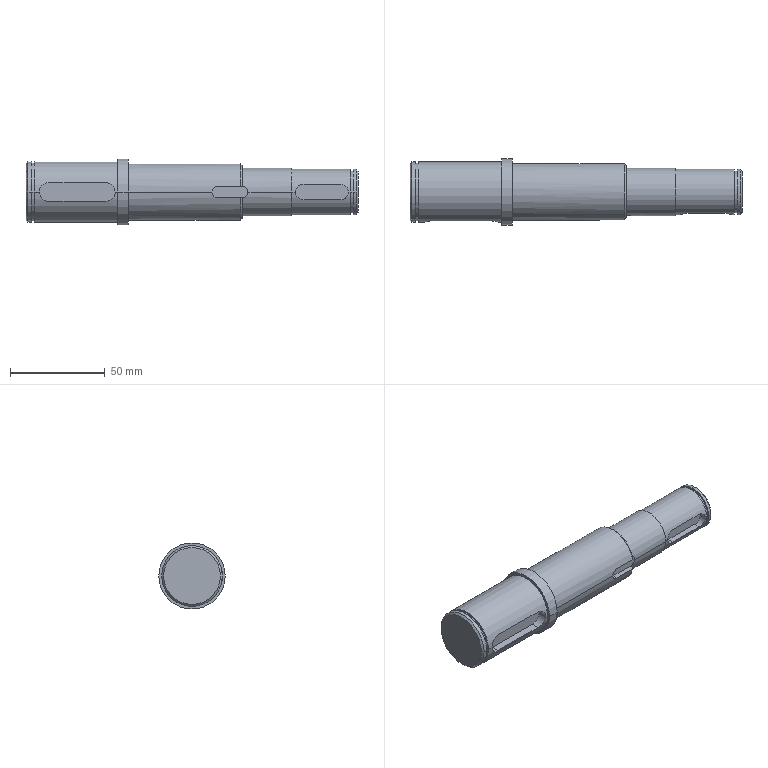Part | SolidWorks | features BaseBody 1 | 1 solid | 51 faces | box 175 x 35 x 35 mm | volume 112132 mm3 | cylinder 25 | plane 19 | cone 7 | commonest cylinder face diameters 24 x4 32 x4 10 x3 6 x2 8 x2 22 x2